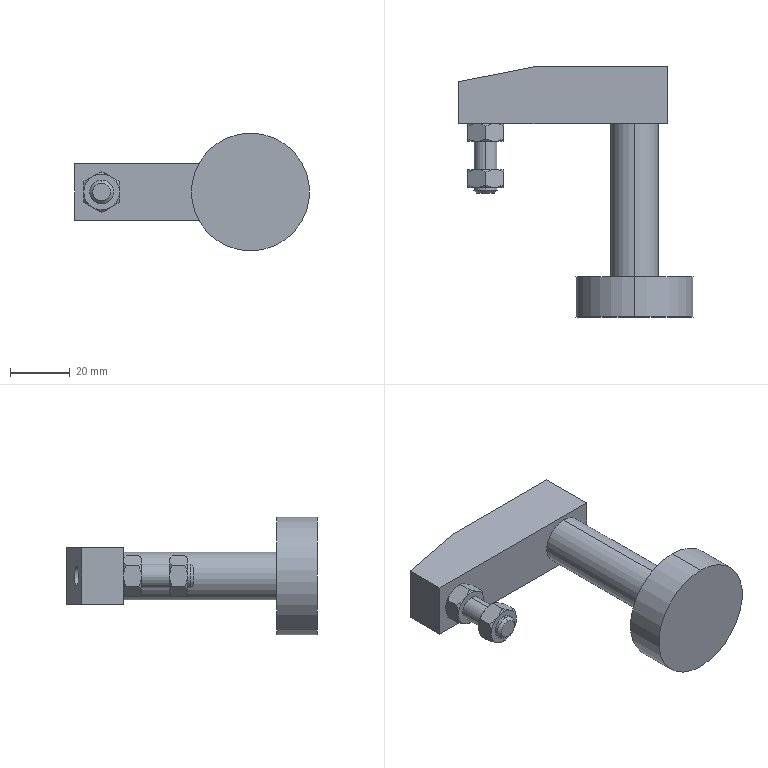Part | SolidWorks | features BaseBody 1 | 1 solid | 76 faces | box 78.8 x 84 x 39.6 mm | volume 52858 mm3 | cone 34 | plane 28 | cylinder 14 | commonest cylinder face diameters 8 x4 6.647 x2 13 x2 14 x2 16 x2 39.6 x2